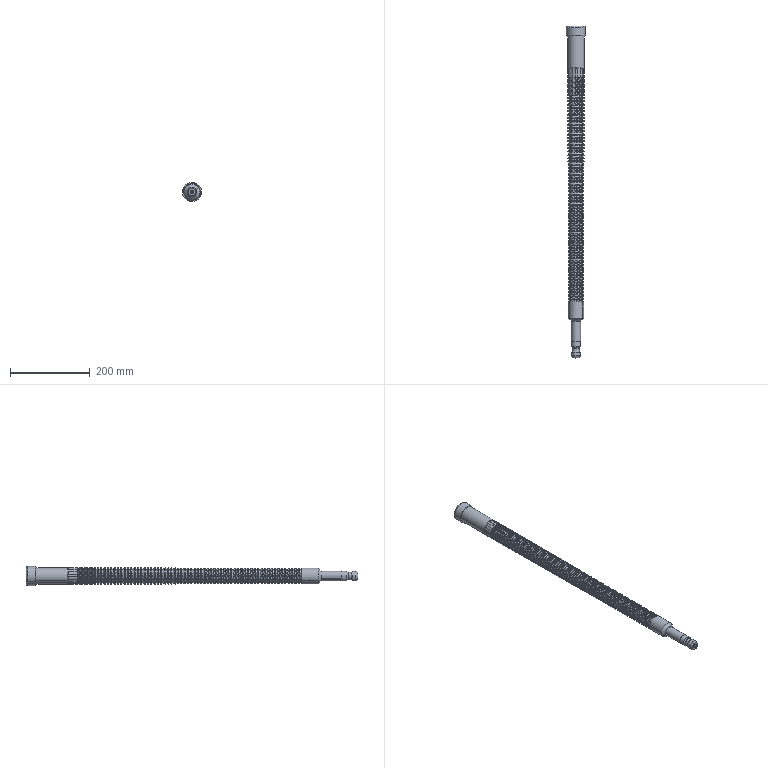Part | STEP file | 2026.6.15-Main Assembly图.sldasm-Part-40 | 1 solid | 4154 faces | volume 819781 mm3 | plane 2028 | cone 1002 | spline 500 | cylinder 426 | torus 198 | commonest cylinder face diameters 38.423 x204 39.244 x192 42 x12 24.5 x4 3.862 x2 9.219 x2